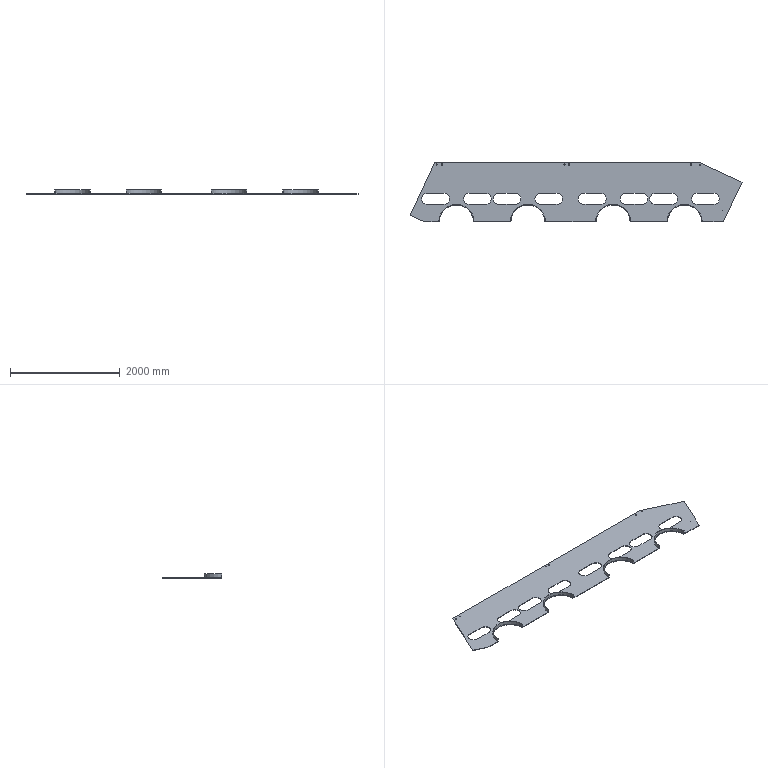Part | STEP file | Side plate_Default<As machined> | 5 solids | 94 faces | box 6040 x 1090 x 73 mm | volume 39402271 mm3 | cylinder 50 | plane 44 | commonest cylinder face diameters 204 x24 22 x8 21 x4 618 x4 628 x4 640 x4